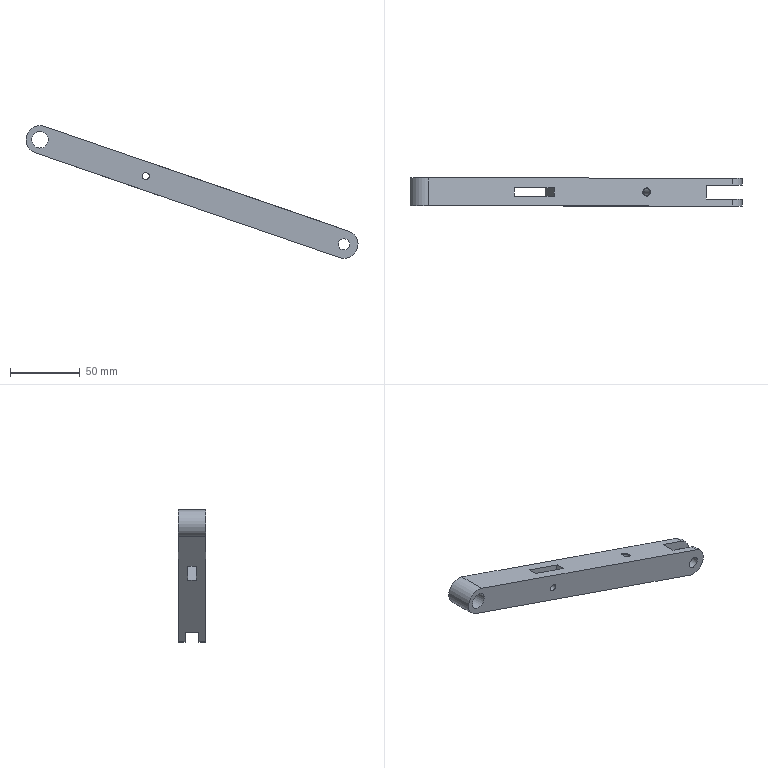Part | STEP file | 冲床-300配套压波_id682_x_t | 1 solid | 22 faces | box 237.457 x 20 x 94.916 mm | volume 85651 mm3 | plane 11 | cylinder 9 | cone 2 | commonest cylinder face diameters 5 x3 20 x3 8 x2 12 x1
STEP:
#1=CARTESIAN_POINT('',(2190.2,-5.,-445.371));
#2=VERTEX_POINT('',#1);
#3=CARTESIAN_POINT('',(2171.291,-5.,-438.856));
#4=VERTEX_POINT('',#3);
#5=CARTESIAN_POINT('',(2038.925,-5.,-393.255));
#6=DIRECTION('',(-0.9455,0.,0.3257));
#7=VECTOR('',#6,1.);
#8=LINE('',#5,#7);
#9=EDGE_CURVE('',#2,#4,#8,.T.);
#10=ORIENTED_EDGE('',*,*,#9,.F.);
#11=CARTESIAN_POINT('',(2190.2,-10.,-445.371));
#12=VERTEX_POINT('',#11);
#13=CARTESIAN_POINT('',(2190.2,-10.,-445.371));
#14=DIRECTION('',(0.,-1.,0.));
#15=VECTOR('',#14,1.);
#16=LINE('',#13,#15);
#17=EDGE_CURVE('',#2,#12,#16,.T.);
#18=ORIENTED_EDGE('',*,*,#17,.T.);
#19=CARTESIAN_POINT('',(1972.743,-10.,-370.455));
#20=VERTEX_POINT('',#19);
#21=CARTESIAN_POINT('',(1958.561,-10.,-365.569));
#22=DIRECTION('',(0.9455,0.,-0.3257));
#23=VECTOR('',#22,1.);
#24=LINE('',#21,#23);
#25=EDGE_CURVE('',#20,#12,#24,.T.);
#26=ORIENTED_EDGE('',*,*,#25,.F.);
#27=CARTESIAN_POINT('',(1972.743,10.,-370.455));
#28=VERTEX_POINT('',#27);
#29=CARTESIAN_POINT('',(1972.743,0.,-370.455));
#30=DIRECTION('',(0.,1.,0.));
#31=VECTOR('',#30,1.);
#32=LINE('',#29,#31);
#33=EDGE_CURVE('',#20,#28,#32,.T.);
#34=ORIENTED_EDGE('',*,*,#33,.T.);
#35=CARTESIAN_POINT('',(2190.2,10.,-445.371));
#36=VERTEX_POINT('',#35);
#37=CARTESIAN_POINT('',(1958.561,10.,-365.569));
#38=DIRECTION('',(0.9455,0.,-0.3257));
#39=VECTOR('',#38,1.);
#40=LINE('',#37,#39);
#41=EDGE_CURVE('',#28,#36,#40,.T.);
#42=ORIENTED_EDGE('',*,*,#41,.T.);
#43=CARTESIAN_POINT('',(2190.2,5.,-445.371));
#44=VERTEX_POINT('',#43);
#45=CARTESIAN_POINT('',(2190.2,-10.,-445.371));
#46=DIRECTION('',(0.,-1.,0.));
#47=VECTOR('',#46,1.);
#48=LINE('',#45,#47);
#49=EDGE_CURVE('',#36,#44,#48,.T.);
#50=ORIENTED_EDGE('',*,*,#49,.T.);
#51=CARTESIAN_POINT('',(2171.291,5.,-438.856));
#52=VERTEX_POINT('',#51);
#53=CARTESIAN_POINT('',(2038.925,5.,-393.255));
#54=DIRECTION('',(0.9455,0.,-0.3257));
#55=VECTOR('',#54,1.);
#56=LINE('',#53,#55);
#57=EDGE_CURVE('',#52,#44,#56,.T.);
#58=ORIENTED_EDGE('',*,*,#57,.F.);
#59=CARTESIAN_POINT('',(2171.291,-10.,-438.856));
#60=DIRECTION('',(0.,1.,0.));
#61=VECTOR('',#60,1.);
#62=LINE('',#59,#61);
#63=EDGE_CURVE('',#4,#52,#62,.T.);
#64=ORIENTED_EDGE('',*,*,#63,.F.);
#65=EDGE_LOOP('',(#10,#18,#26,#34,#42,#50,#58,#64));
#66=FACE_BOUND('',#65,.T.);
#67=CARTESIAN_POINT('',(2062.562,3.15,-401.398));
#68=VERTEX_POINT('',#67);
#69=CARTESIAN_POINT('',(2062.562,-3.15,-401.398));
#70=VERTEX_POINT('',#69);
#71=CARTESIAN_POINT('',(2062.562,-3.1,-401.398));
#72=DIRECTION('',(0.,-1.,0.));
#73=VECTOR('',#72,1.);
#74=LINE('',#71,#73);
#75=EDGE_CURVE('',#68,#70,#74,.T.);
#76=ORIENTED_EDGE('',*,*,#75,.F.);
#77=CARTESIAN_POINT('',(2034.198,3.15,-391.627));
#78=VERTEX_POINT('',#77);
#79=CARTESIAN_POINT('',(1977.47,3.15,-372.083));
#80=DIRECTION('',(0.9455,0.,-0.3257));
#81=VECTOR('',#80,1.);
#82=LINE('',#79,#81);
#83=EDGE_CURVE('',#78,#68,#82,.T.);
#84=ORIENTED_EDGE('',*,*,#83,.F.);
#85=CARTESIAN_POINT('',(2034.198,-3.15,-391.627));
#86=VERTEX_POINT('',#85);
#87=CARTESIAN_POINT('',(2034.198,-10.,-391.627));
#88=DIRECTION('',(0.,-1.,0.));
#89=VECTOR('',#88,1.);
#90=LINE('',#87,#89);
#91=EDGE_CURVE('',#78,#86,#90,.T.);
#92=ORIENTED_EDGE('',*,*,#91,.T.);
#93=CARTESIAN_POINT('',(1977.47,-3.15,-372.083));
#94=DIRECTION('',(-0.9455,0.,0.3257));
#95=VECTOR('',#94,1.);
#96=LINE('',#93,#95);
#97=EDGE_CURVE('',#70,#86,#96,.T.);
#98=ORIENTED_EDGE('',*,*,#97,.F.);
#99=EDGE_LOOP('',(#76,#84,#92,#98));
#100=FACE_BOUND('',#99,.T.);
#101=CARTESIAN_POINT('',(1958.561,-10.,-365.569));
#102=DIRECTION('',(0.3257,0.,0.9455));
#103=DIRECTION('',(0.9455,0.,-0.3257));
#104=AXIS2_PLACEMENT_3D('',#101,#102,#103);
#105=PLANE('',#104);
#106=ADVANCED_FACE('',(#66,#100),#105,.F.);
#107=CARTESIAN_POINT('',(2132.423,0.,-404.312));
#108=VERTEX_POINT('',#107);
#109=CARTESIAN_POINT('',(2135.259,0.,-405.289));
#110=DIRECTION('',(-0.3257,0.,-0.9455));
#111=DIRECTION('',(-0.9455,0.,0.3257));
#112=AXIS2_PLACEMENT_3D('',#109,#110,#111);
#113=CIRCLE('',#112,3.);
#114=EDGE_CURVE('',#108,#108,#113,.T.);
#115=ORIENTED_EDGE('',*,*,#114,.T.);
#116=EDGE_LOOP('',(#115));
#117=FACE_BOUND('',#116,.T.);
#118=CARTESIAN_POINT('',(2177.805,-5.,-419.947));
#119=VERTEX_POINT('',#118);
#120=CARTESIAN_POINT('',(2196.714,-5.,-426.461));
#121=VERTEX_POINT('',#120);
#122=CARTESIAN_POINT('',(2187.26,-5.,-423.204));
#123=DIRECTION('',(0.9455,0.,-0.3257));
#124=VECTOR('',#123,1.);
#125=LINE('',#122,#124);
#126=EDGE_CURVE('',#119,#121,#125,.T.);
#127=ORIENTED_EDGE('',*,*,#126,.F.);
#128=CARTESIAN_POINT('',(2177.805,5.,-419.947));
#129=VERTEX_POINT('',#128);
#130=CARTESIAN_POINT('',(2177.805,-10.,-419.947));
#131=DIRECTION('',(0.,-1.,0.));
#132=VECTOR('',#131,1.);
#133=LINE('',#130,#132);
#134=EDGE_CURVE('',#129,#119,#133,.T.);
#135=ORIENTED_EDGE('',*,*,#134,.F.);
#136=CARTESIAN_POINT('',(2196.714,5.,-426.461));
#137=VERTEX_POINT('',#136);
#138=CARTESIAN_POINT('',(2187.26,5.,-423.204));
#139=DIRECTION('',(-0.9455,0.,0.3257));
#140=VECTOR('',#139,1.);
#141=LINE('',#138,#140);
#142=EDGE_CURVE('',#137,#129,#141,.T.);
#143=ORIENTED_EDGE('',*,*,#142,.F.);
#144=CARTESIAN_POINT('',(2196.714,10.,-426.461));
#145=VERTEX_POINT('',#144);
#146=CARTESIAN_POINT('',(2196.714,-10.,-426.461));
#147=DIRECTION('',(0.,1.,0.));
#148=VECTOR('',#147,1.);
#149=LINE('',#146,#148);
#150=EDGE_CURVE('',#137,#145,#149,.T.);
#151=ORIENTED_EDGE('',*,*,#150,.T.);
#152=CARTESIAN_POINT('',(1979.257,10.,-351.545));
#153=VERTEX_POINT('',#152);
#154=CARTESIAN_POINT('',(2106.895,10.,-395.518));
#155=DIRECTION('',(-0.9455,0.,0.3257));
#156=VECTOR('',#155,1.);
#157=LINE('',#154,#156);
#158=EDGE_CURVE('',#145,#153,#157,.T.);
#159=ORIENTED_EDGE('',*,*,#158,.T.);
#160=CARTESIAN_POINT('',(1979.257,-10.,-351.545));
#161=VERTEX_POINT('',#160);
#162=CARTESIAN_POINT('',(1979.257,0.,-351.545));
#163=DIRECTION('',(0.,-1.,0.));
#164=VECTOR('',#163,1.);
#165=LINE('',#162,#164);
#166=EDGE_CURVE('',#153,#161,#165,.T.);
#167=ORIENTED_EDGE('',*,*,#166,.T.);
#168=CARTESIAN_POINT('',(2196.714,-10.,-426.461));
#169=VERTEX_POINT('',#168);
#170=CARTESIAN_POINT('',(2106.895,-10.,-395.518));
#171=DIRECTION('',(-0.9455,0.,0.3257));
#172=VECTOR('',#171,1.);
#173=LINE('',#170,#172);
#174=EDGE_CURVE('',#169,#161,#173,.T.);
#175=ORIENTED_EDGE('',*,*,#174,.F.);
#176=CARTESIAN_POINT('',(2196.714,-10.,-426.461));
#177=DIRECTION('',(0.,1.,0.));
#178=VECTOR('',#177,1.);
#179=LINE('',#176,#178);
#180=EDGE_CURVE('',#169,#121,#179,.T.);
#181=ORIENTED_EDGE('',*,*,#180,.T.);
#182=EDGE_LOOP('',(#127,#135,#143,#151,#159,#167,#175,#181));
#183=FACE_BOUND('',#182,.T.);
#184=CARTESIAN_POINT('',(2040.712,3.15,-372.717));
#185=VERTEX_POINT('',#184);
#186=CARTESIAN_POINT('',(2069.076,3.15,-382.489));
#187=VERTEX_POINT('',#186);
#188=CARTESIAN_POINT('',(2066.439,3.15,-381.58));
#189=DIRECTION('',(0.9455,0.,-0.3257));
#190=VECTOR('',#189,1.);
#191=LINE('',#188,#190);
#192=EDGE_CURVE('',#185,#187,#191,.T.);
#193=ORIENTED_EDGE('',*,*,#192,.T.);
#194=CARTESIAN_POINT('',(2069.076,-3.15,-382.489));
#195=VERTEX_POINT('',#194);
#196=CARTESIAN_POINT('',(2069.076,-10.,-382.489));
#197=DIRECTION('',(0.,-1.,0.));
#198=VECTOR('',#197,1.);
#199=LINE('',#196,#198);
#200=EDGE_CURVE('',#187,#195,#199,.T.);
#201=ORIENTED_EDGE('',*,*,#200,.T.);
#202=CARTESIAN_POINT('',(2040.712,-3.15,-372.717));
#203=VERTEX_POINT('',#202);
#204=CARTESIAN_POINT('',(2066.439,-3.15,-381.58));
#205=DIRECTION('',(-0.9455,0.,0.3257));
#206=VECTOR('',#205,1.);
#207=LINE('',#204,#206);
#208=EDGE_CURVE('',#195,#203,#207,.T.);
#209=ORIENTED_EDGE('',*,*,#208,.T.);
#210=CARTESIAN_POINT('',(2040.712,-10.,-372.717));
#211=DIRECTION('',(0.,1.,0.));
#212=VECTOR('',#211,1.);
#213=LINE('',#210,#212);
#214=EDGE_CURVE('',#203,#185,#213,.T.);
#215=ORIENTED_EDGE('',*,*,#214,.T.);
#216=EDGE_LOOP('',(#193,#201,#209,#215));
#217=FACE_BOUND('',#216,.T.);
#218=CARTESIAN_POINT('',(2106.895,-10.,-395.518));
#219=DIRECTION('',(-0.3257,0.,-0.9455));
#220=DIRECTION('',(-0.9455,0.,0.3257));
#221=AXIS2_PLACEMENT_3D('',#218,#219,#220);
#222=PLANE('',#221);
#223=ADVANCED_FACE('',(#117,#183,#217),#222,.F.);
#224=CARTESIAN_POINT('',(2050.584,-3.15,-384.79));
#225=VERTEX_POINT('',#224);
#226=CARTESIAN_POINT('',(2051.637,-3.15,-387.058));
#227=DIRECTION('',(0.,-1.,0.));
#228=DIRECTION('',(-0.4213,0.,0.9069));
#229=AXIS2_PLACEMENT_3D('',#226,#227,#228);
#230=CIRCLE('',#229,2.5);
#231=EDGE_CURVE('',#225,#225,#230,.T.);
#232=ORIENTED_EDGE('',*,*,#231,.F.);
#233=EDGE_LOOP('',(#232));
#234=FACE_BOUND('',#233,.T.);
#235=CARTESIAN_POINT('',(2050.064,-10.,-389.));
#236=VERTEX_POINT('',#235);
#237=CARTESIAN_POINT('',(2051.637,-10.,-387.058));
#238=DIRECTION('',(0.,1.,0.));
#239=DIRECTION('',(-0.6294,0.,-0.777));
#240=AXIS2_PLACEMENT_3D('',#237,#238,#239);
#241=CIRCLE('',#240,2.5);
#242=EDGE_CURVE('',#236,#236,#241,.T.);
#243=ORIENTED_EDGE('',*,*,#242,.F.);
#244=EDGE_LOOP('',(#243));
#245=FACE_BOUND('',#244,.T.);
#246=CARTESIAN_POINT('',(2051.637,-45.,-387.058));
#247=DIRECTION('',(0.,1.,0.));
#248=DIRECTION('',(0.6294,0.,0.777));
#249=AXIS2_PLACEMENT_3D('',#246,#247,#248);
#250=CYLINDRICAL_SURFACE('',#249,2.5);
#251=ADVANCED_FACE('',(#234,#245),#250,.F.);
#252=ORIENTED_EDGE('',*,*,#150,.F.);
#253=CARTESIAN_POINT('',(2193.457,5.,-435.916));
#254=DIRECTION('',(0.,1.,0.));
#255=DIRECTION('',(-0.3257,0.,-0.9455));
#256=AXIS2_PLACEMENT_3D('',#253,#254,#255);
#257=CIRCLE('',#256,10.);
#258=EDGE_CURVE('',#137,#44,#257,.T.);
#259=ORIENTED_EDGE('',*,*,#258,.T.);
#260=ORIENTED_EDGE('',*,*,#49,.F.);
#261=CARTESIAN_POINT('',(2193.457,10.,-435.916));
#262=DIRECTION('',(0.,1.,0.));
#263=DIRECTION('',(-0.3257,0.,-0.9455));
#264=AXIS2_PLACEMENT_3D('',#261,#262,#263);
#265=CIRCLE('',#264,10.);
#266=EDGE_CURVE('',#145,#36,#265,.T.);
#267=ORIENTED_EDGE('',*,*,#266,.F.);
#268=EDGE_LOOP('',(#252,#259,#260,#267));
#269=FACE_OUTER_BOUND('',#268,.T.);
#270=CARTESIAN_POINT('',(2193.457,-10.,-435.916));
#271=DIRECTION('',(0.,1.,0.));
#272=DIRECTION('',(0.3257,0.,0.9455));
#273=AXIS2_PLACEMENT_3D('',#270,#271,#272);
#274=CYLINDRICAL_SURFACE('',#273,10.);
#275=ADVANCED_FACE('',(#269),#274,.T.);
#276=ORIENTED_EDGE('',*,*,#17,.F.);
#277=CARTESIAN_POINT('',(2193.457,-5.,-435.916));
#278=DIRECTION('',(0.,-1.,0.));
#279=DIRECTION('',(0.3257,0.,0.9455));
#280=AXIS2_PLACEMENT_3D('',#277,#278,#279);
#281=CIRCLE('',#280,10.);
#282=EDGE_CURVE('',#2,#121,#281,.T.);
#283=ORIENTED_EDGE('',*,*,#282,.T.);
#284=ORIENTED_EDGE('',*,*,#180,.F.);
#285=CARTESIAN_POINT('',(2193.457,-10.,-435.916));
#286=DIRECTION('',(0.,-1.,0.));
#287=DIRECTION('',(-0.3257,0.,-0.9455));
#288=AXIS2_PLACEMENT_3D('',#285,#286,#287);
#289=CIRCLE('',#288,10.);
#290=EDGE_CURVE('',#12,#169,#289,.T.);
#291=ORIENTED_EDGE('',*,*,#290,.F.);
#292=EDGE_LOOP('',(#276,#283,#284,#291));
#293=FACE_OUTER_BOUND('',#292,.T.);
#294=CARTESIAN_POINT('',(2193.457,-10.,-435.916));
#295=DIRECTION('',(0.,1.,0.));
#296=DIRECTION('',(0.3257,0.,0.9455));
#297=AXIS2_PLACEMENT_3D('',#294,#295,#296);
#298=CYLINDRICAL_SURFACE('',#297,10.);
#299=ADVANCED_FACE('',(#293),#298,.T.);
#300=CARTESIAN_POINT('',(2192.154,-10.,-439.698));
#301=VERTEX_POINT('',#300);
#302=CARTESIAN_POINT('',(2193.457,-10.,-435.916));
#303=DIRECTION('',(0.,1.,0.));
#304=DIRECTION('',(-0.3257,0.,-0.9455));
#305=AXIS2_PLACEMENT_3D('',#302,#303,#304);
#306=CIRCLE('',#305,4.);
#307=EDGE_CURVE('',#301,#301,#306,.T.);
#308=ORIENTED_EDGE('',*,*,#307,.F.);
#309=EDGE_LOOP('',(#308));
#310=FACE_BOUND('',#309,.T.);
#311=CARTESIAN_POINT('',(2194.76,-5.,-432.134));
#312=VERTEX_POINT('',#311);
#313=CARTESIAN_POINT('',(2193.457,-5.,-435.916));
#314=DIRECTION('',(0.,-1.,0.));
#315=DIRECTION('',(0.3257,0.,0.9455));
#316=AXIS2_PLACEMENT_3D('',#313,#314,#315);
#317=CIRCLE('',#316,4.);
#318=EDGE_CURVE('',#312,#312,#317,.T.);
#319=ORIENTED_EDGE('',*,*,#318,.F.);
#320=EDGE_LOOP('',(#319));
#321=FACE_BOUND('',#320,.T.);
#322=CARTESIAN_POINT('',(2193.457,-10.,-435.916));
#323=DIRECTION('',(0.,1.,0.));
#324=DIRECTION('',(0.3257,0.,0.9455));
#325=AXIS2_PLACEMENT_3D('',#322,#323,#324);
#326=CYLINDRICAL_SURFACE('',#325,4.);
#327=ADVANCED_FACE('',(#310,#321),#326,.F.);
#328=CARTESIAN_POINT('',(2192.154,10.,-439.698));
#329=VERTEX_POINT('',#328);
#330=CARTESIAN_POINT('',(2193.457,10.,-435.916));
#331=DIRECTION('',(0.,-1.,0.));
#332=DIRECTION('',(-0.3257,0.,-0.9455));
#333=AXIS2_PLACEMENT_3D('',#330,#331,#332);
#334=CIRCLE('',#333,4.);
#335=EDGE_CURVE('',#329,#329,#334,.T.);
#336=ORIENTED_EDGE('',*,*,#335,.F.);
#337=EDGE_LOOP('',(#336));
#338=FACE_BOUND('',#337,.T.);
#339=CARTESIAN_POINT('',(2192.154,5.,-439.698));
#340=VERTEX_POINT('',#339);
#341=CARTESIAN_POINT('',(2193.457,5.,-435.916));
#342=DIRECTION('',(0.,1.,0.));
#343=DIRECTION('',(-0.3257,0.,-0.9455));
#344=AXIS2_PLACEMENT_3D('',#341,#342,#343);
#345=CIRCLE('',#344,4.);
#346=EDGE_CURVE('',#340,#340,#345,.T.);
#347=ORIENTED_EDGE('',*,*,#346,.F.);
#348=EDGE_LOOP('',(#347));
#349=FACE_BOUND('',#348,.T.);
#350=CARTESIAN_POINT('',(2193.457,-10.,-435.916));
#351=DIRECTION('',(0.,1.,0.));
#352=DIRECTION('',(0.3257,0.,0.9455));
#353=AXIS2_PLACEMENT_3D('',#350,#351,#352);
#354=CYLINDRICAL_SURFACE('',#353,4.);
#355=ADVANCED_FACE('',(#338,#349),#354,.F.);
#356=ORIENTED_EDGE('',*,*,#242,.T.);
#357=EDGE_LOOP('',(#356));
#358=FACE_BOUND('',#357,.T.);
#359=CARTESIAN_POINT('',(1976.,-10.,-367.));
#360=VERTEX_POINT('',#359);
#361=CARTESIAN_POINT('',(1976.,-10.,-361.));
#362=DIRECTION('',(0.,1.,0.));
#363=DIRECTION('',(0.,0.,-1.));
#364=AXIS2_PLACEMENT_3D('',#361,#362,#363);
#365=CIRCLE('',#364,6.);
#366=EDGE_CURVE('',#360,#360,#365,.T.);
#367=ORIENTED_EDGE('',*,*,#366,.T.);
#368=EDGE_LOOP('',(#367));
#369=FACE_BOUND('',#368,.T.);
#370=ORIENTED_EDGE('',*,*,#307,.T.);
#371=EDGE_LOOP('',(#370));
#372=FACE_BOUND('',#371,.T.);
#373=ORIENTED_EDGE('',*,*,#25,.T.);
#374=ORIENTED_EDGE('',*,*,#290,.T.);
#375=ORIENTED_EDGE('',*,*,#174,.T.);
#376=CARTESIAN_POINT('',(1976.,-10.,-361.));
#377=DIRECTION('',(0.,-1.,0.));
#378=DIRECTION('',(0.4213,0.,-0.9069));
#379=AXIS2_PLACEMENT_3D('',#376,#377,#378);
#380=CIRCLE('',#379,10.);
#381=EDGE_CURVE('',#161,#20,#380,.T.);
#382=ORIENTED_EDGE('',*,*,#381,.T.);
#383=EDGE_LOOP('',(#373,#374,#375,#382));
#384=FACE_BOUND('',#383,.T.);
#385=CARTESIAN_POINT('',(184.727,-10.,507.573));
#386=DIRECTION('',(0.,-1.,0.));
#387=DIRECTION('',(-0.3257,0.,-0.9455));
#388=AXIS2_PLACEMENT_3D('',#385,#386,#387);
#389=PLANE('',#388);
#390=ADVANCED_FACE('',(#358,#369,#372,#384),#389,.T.);
#391=CARTESIAN_POINT('',(2050.064,10.,-389.));
#392=VERTEX_POINT('',#391);
#393=CARTESIAN_POINT('',(2051.637,10.,-387.058));
#394=DIRECTION('',(0.,1.,0.));
#395=DIRECTION('',(-0.6294,0.,-0.777));
#396=AXIS2_PLACEMENT_3D('',#393,#394,#395);
#397=CIRCLE('',#396,2.5);
#398=EDGE_CURVE('',#392,#392,#397,.T.);
#399=ORIENTED_EDGE('',*,*,#398,.F.);
#400=EDGE_LOOP('',(#399));
#401=FACE_BOUND('',#400,.T.);
#402=CARTESIAN_POINT('',(1976.,10.,-367.));
#403=VERTEX_POINT('',#402);
#404=CARTESIAN_POINT('',(1976.,10.,-361.));
#405=DIRECTION('',(0.,1.,0.));
#406=DIRECTION('',(0.,0.,-1.));
#407=AXIS2_PLACEMENT_3D('',#404,#405,#406);
#408=CIRCLE('',#407,6.);
#409=EDGE_CURVE('',#403,#403,#408,.T.);
#410=ORIENTED_EDGE('',*,*,#409,.F.);
#411=EDGE_LOOP('',(#410));
#412=FACE_BOUND('',#411,.T.);
#413=ORIENTED_EDGE('',*,*,#335,.T.);
#414=EDGE_LOOP('',(#413));
#415=FACE_BOUND('',#414,.T.);
#416=ORIENTED_EDGE('',*,*,#266,.T.);
#417=ORIENTED_EDGE('',*,*,#41,.F.);
#418=CARTESIAN_POINT('',(1976.,10.,-361.));
#419=DIRECTION('',(0.,1.,0.));
#420=DIRECTION('',(0.4213,0.,-0.9069));
#421=AXIS2_PLACEMENT_3D('',#418,#419,#420);
#422=CIRCLE('',#421,10.);
#423=EDGE_CURVE('',#28,#153,#422,.T.);
#424=ORIENTED_EDGE('',*,*,#423,.T.);
#425=ORIENTED_EDGE('',*,*,#158,.F.);
#426=EDGE_LOOP('',(#416,#417,#424,#425));
#427=FACE_BOUND('',#426,.T.);
#428=CARTESIAN_POINT('',(184.727,10.,507.573));
#429=DIRECTION('',(0.,-1.,0.));
#430=DIRECTION('',(-0.3257,0.,-0.9455));
#431=AXIS2_PLACEMENT_3D('',#428,#429,#430);
#432=PLANE('',#431);
#433=ADVANCED_FACE('',(#401,#412,#415,#427),#432,.F.);
#434=ORIENTED_EDGE('',*,*,#423,.F.);
#435=ORIENTED_EDGE('',*,*,#33,.F.);
#436=ORIENTED_EDGE('',*,*,#381,.F.);
#437=ORIENTED_EDGE('',*,*,#166,.F.);
#438=EDGE_LOOP('',(#434,#435,#436,#437));
#439=FACE_OUTER_BOUND('',#438,.T.);
#440=CARTESIAN_POINT('',(1976.,-2.,-361.));
#441=DIRECTION('',(0.,-1.,0.));
#442=DIRECTION('',(0.4213,0.,-0.9069));
#443=AXIS2_PLACEMENT_3D('',#440,#441,#442);
#444=CYLINDRICAL_SURFACE('',#443,10.);
#445=ADVANCED_FACE('',(#439),#444,.T.);
#446=ORIENTED_EDGE('',*,*,#366,.F.);
#447=EDGE_LOOP('',(#446));
#448=FACE_BOUND('',#447,.T.);
#449=ORIENTED_EDGE('',*,*,#409,.T.);
#450=EDGE_LOOP('',(#449));
#451=FACE_BOUND('',#450,.T.);
#452=CARTESIAN_POINT('',(1976.,32.85,-361.));
#453=DIRECTION('',(0.,-1.,0.));
#454=DIRECTION('',(-0.3257,0.,-0.9455));
#455=AXIS2_PLACEMENT_3D('',#452,#453,#454);
#456=CYLINDRICAL_SURFACE('',#455,6.);
#457=ADVANCED_FACE('',(#448,#451),#456,.F.);
#458=ORIENTED_EDGE('',*,*,#63,.T.);
#459=CARTESIAN_POINT('',(2184.319,5.,-401.038));
#460=DIRECTION('',(0.3257,0.,0.9455));
#461=VECTOR('',#460,1.);
#462=LINE('',#459,#461);
#463=EDGE_CURVE('',#52,#129,#462,.T.);
#464=ORIENTED_EDGE('',*,*,#463,.T.);
#465=ORIENTED_EDGE('',*,*,#134,.T.);
#466=CARTESIAN_POINT('',(2184.319,-5.,-401.038));
#467=DIRECTION('',(0.3257,0.,0.9455));
#468=VECTOR('',#467,1.);
#469=LINE('',#466,#468);
#470=EDGE_CURVE('',#4,#119,#469,.T.);
#471=ORIENTED_EDGE('',*,*,#470,.F.);
#472=EDGE_LOOP('',(#458,#464,#465,#471));
#473=FACE_OUTER_BOUND('',#472,.T.);
#474=CARTESIAN_POINT('',(2184.319,5.,-401.038));
#475=DIRECTION('',(0.9455,0.,-0.3257));
#476=DIRECTION('',(-0.3257,0.,-0.9455));
#477=AXIS2_PLACEMENT_3D('',#474,#475,#476);
#478=PLANE('',#477);
#479=ADVANCED_FACE('',(#473),#478,.T.);
#480=ORIENTED_EDGE('',*,*,#318,.T.);
#481=EDGE_LOOP('',(#480));
#482=FACE_BOUND('',#481,.T.);
#483=ORIENTED_EDGE('',*,*,#9,.T.);
#484=ORIENTED_EDGE('',*,*,#470,.T.);
#485=ORIENTED_EDGE('',*,*,#126,.T.);
#486=ORIENTED_EDGE('',*,*,#282,.F.);
#487=EDGE_LOOP('',(#483,#484,#485,#486));
#488=FACE_BOUND('',#487,.T.);
#489=CARTESIAN_POINT('',(2184.319,-5.,-401.038));
#490=DIRECTION('',(0.,1.,0.));
#491=DIRECTION('',(0.3257,0.,0.9455));
#492=AXIS2_PLACEMENT_3D('',#489,#490,#491);
#493=PLANE('',#492);
#494=ADVANCED_FACE('',(#482,#488),#493,.T.);
#495=ORIENTED_EDGE('',*,*,#346,.T.);
#496=EDGE_LOOP('',(#495));
#497=FACE_BOUND('',#496,.T.);
#498=ORIENTED_EDGE('',*,*,#57,.T.);
#499=ORIENTED_EDGE('',*,*,#258,.F.);
#500=ORIENTED_EDGE('',*,*,#142,.T.);
#501=ORIENTED_EDGE('',*,*,#463,.F.);
#502=EDGE_LOOP('',(#498,#499,#500,#501));
#503=FACE_BOUND('',#502,.T.);
#504=CARTESIAN_POINT('',(2223.333,5.,-414.478));
#505=DIRECTION('',(0.,-1.,0.));
#506=DIRECTION('',(-0.3257,0.,-0.9455));
#507=AXIS2_PLACEMENT_3D('',#504,#505,#506);
#508=PLANE('',#507);
#509=ADVANCED_FACE('',(#497,#503),#508,.T.);
#510=CARTESIAN_POINT('',(2052.69,3.15,-389.325));
#511=VERTEX_POINT('',#510);
#512=CARTESIAN_POINT('',(2051.637,3.15,-387.058));
#513=DIRECTION('',(0.,1.,0.));
#514=DIRECTION('',(0.4213,0.,-0.9069));
#515=AXIS2_PLACEMENT_3D('',#512,#513,#514);
#516=CIRCLE('',#515,2.5);
#517=EDGE_CURVE('',#511,#511,#516,.T.);
#518=ORIENTED_EDGE('',*,*,#517,.F.);
#519=EDGE_LOOP('',(#518));
#520=FACE_BOUND('',#519,.T.);
#521=ORIENTED_EDGE('',*,*,#398,.T.);
#522=EDGE_LOOP('',(#521));
#523=FACE_BOUND('',#522,.T.);
#524=CARTESIAN_POINT('',(2051.637,-45.,-387.058));
#525=DIRECTION('',(0.,1.,0.));
#526=DIRECTION('',(0.6294,0.,0.777));
#527=AXIS2_PLACEMENT_3D('',#524,#525,#526);
#528=CYLINDRICAL_SURFACE('',#527,2.5);
#529=ADVANCED_FACE('',(#520,#523),#528,.F.);
#530=CARTESIAN_POINT('',(2128.987,0.,-415.821));
#531=VERTEX_POINT('',#530);
#532=CARTESIAN_POINT('',(2131.35,0.,-416.635));
#533=DIRECTION('',(0.3257,0.,0.9455));
#534=DIRECTION('',(-0.9455,0.,0.3257));
#535=AXIS2_PLACEMENT_3D('',#532,#533,#534);
#536=CIRCLE('',#535,2.5);
#537=EDGE_CURVE('',#531,#531,#536,.T.);
#538=ORIENTED_EDGE('',*,*,#537,.T.);
#539=EDGE_LOOP('',(#538));
#540=FACE_BOUND('',#539,.T.);
#541=CARTESIAN_POINT('',(2130.861,0.,-418.055));
#542=VERTEX_POINT('',#541);
#543=VERTEX_LOOP('',#542);
#544=FACE_BOUND('',#543,.T.);
#545=CARTESIAN_POINT('',(2131.35,0.,-416.635));
#546=DIRECTION('',(0.3257,0.,0.9455));
#547=DIRECTION('',(0.9455,0.,-0.3257));
#548=AXIS2_PLACEMENT_3D('',#545,#546,#547);
#549=CONICAL_SURFACE('',#548,2.5,59.);
#550=ADVANCED_FACE('',(#540,#544),#549,.F.);
#551=CARTESIAN_POINT('',(2132.733,0.,-404.948));
#552=VERTEX_POINT('',#551);
#553=CARTESIAN_POINT('',(2135.096,0.,-405.762));
#554=DIRECTION('',(0.3257,0.,0.9455));
#555=DIRECTION('',(-0.9455,0.,0.3257));
#556=AXIS2_PLACEMENT_3D('',#553,#554,#555);
#557=CIRCLE('',#556,2.5);
#558=EDGE_CURVE('',#552,#552,#557,.T.);
#559=ORIENTED_EDGE('',*,*,#558,.T.);
#560=EDGE_LOOP('',(#559));
#561=FACE_BOUND('',#560,.T.);
#562=ORIENTED_EDGE('',*,*,#537,.F.);
#563=EDGE_LOOP('',(#562));
#564=FACE_BOUND('',#563,.T.);
#565=CARTESIAN_POINT('',(2135.259,0.,-405.289));
#566=DIRECTION('',(-0.3257,0.,-0.9455));
#567=DIRECTION('',(-0.9455,0.,0.3257));
#568=AXIS2_PLACEMENT_3D('',#565,#566,#567);
#569=CYLINDRICAL_SURFACE('',#568,2.5);
#570=ADVANCED_FACE('',(#561,#564),#569,.F.);
#571=ORIENTED_EDGE('',*,*,#558,.F.);
#572=EDGE_LOOP('',(#571));
#573=FACE_BOUND('',#572,.T.);
#574=ORIENTED_EDGE('',*,*,#114,.F.);
#575=EDGE_LOOP('',(#574));
#576=FACE_BOUND('',#575,.T.);
#577=CARTESIAN_POINT('',(2135.259,0.,-405.289));
#578=DIRECTION('',(0.3257,0.,0.9455));
#579=DIRECTION('',(0.9455,0.,-0.3257));
#580=AXIS2_PLACEMENT_3D('',#577,#578,#579);
#581=CONICAL_SURFACE('',#580,3.,45.);
#582=ADVANCED_FACE('',(#573,#576),#581,.F.);
#583=ORIENTED_EDGE('',*,*,#517,.T.);
#584=EDGE_LOOP('',(#583));
#585=FACE_BOUND('',#584,.T.);
#586=ORIENTED_EDGE('',*,*,#192,.F.);
#587=CARTESIAN_POINT('',(2034.489,3.15,-390.781));
#588=DIRECTION('',(-0.3257,0.,-0.9455));
#589=VECTOR('',#588,1.);
#590=LINE('',#587,#589);
#591=EDGE_CURVE('',#185,#78,#590,.T.);
#592=ORIENTED_EDGE('',*,*,#591,.T.);
#593=ORIENTED_EDGE('',*,*,#83,.T.);
#594=CARTESIAN_POINT('',(2062.853,3.15,-400.553));
#595=DIRECTION('',(0.3257,0.,0.9455));
#596=VECTOR('',#595,1.);
#597=LINE('',#594,#596);
#598=EDGE_CURVE('',#68,#187,#597,.T.);
#599=ORIENTED_EDGE('',*,*,#598,.T.);
#600=EDGE_LOOP('',(#586,#592,#593,#599));
#601=FACE_BOUND('',#600,.T.);
#602=CARTESIAN_POINT('',(2060.215,3.15,-399.644));
#603=DIRECTION('',(0.,-1.,0.));
#604=DIRECTION('',(0.1921,0.,-0.9814));
#605=AXIS2_PLACEMENT_3D('',#602,#603,#604);
#606=PLANE('',#605);
#607=ADVANCED_FACE('',(#585,#601),#606,.T.);
#608=ORIENTED_EDGE('',*,*,#231,.T.);
#609=EDGE_LOOP('',(#608));
#610=FACE_BOUND('',#609,.T.);
#611=ORIENTED_EDGE('',*,*,#97,.T.);
#612=CARTESIAN_POINT('',(2034.489,-3.15,-390.781));
#613=DIRECTION('',(0.3257,0.,0.9455));
#614=VECTOR('',#613,1.);
#615=LINE('',#612,#614);
#616=EDGE_CURVE('',#86,#203,#615,.T.);
#617=ORIENTED_EDGE('',*,*,#616,.T.);
#618=ORIENTED_EDGE('',*,*,#208,.F.);
#619=CARTESIAN_POINT('',(2062.853,-3.15,-400.553));
#620=DIRECTION('',(-0.3257,0.,-0.9455));
#621=VECTOR('',#620,1.);
#622=LINE('',#619,#621);
#623=EDGE_CURVE('',#195,#70,#622,.T.);
#624=ORIENTED_EDGE('',*,*,#623,.T.);
#625=EDGE_LOOP('',(#611,#617,#618,#624));
#626=FACE_BOUND('',#625,.T.);
#627=CARTESIAN_POINT('',(2060.215,-3.15,-399.644));
#628=DIRECTION('',(0.,1.,0.));
#629=DIRECTION('',(-0.1921,0.,0.9814));
#630=AXIS2_PLACEMENT_3D('',#627,#628,#629);
#631=PLANE('',#630);
#632=ADVANCED_FACE('',(#610,#626),#631,.T.);
#633=ORIENTED_EDGE('',*,*,#616,.F.);
#634=ORIENTED_EDGE('',*,*,#91,.F.);
#635=ORIENTED_EDGE('',*,*,#591,.F.);
#636=ORIENTED_EDGE('',*,*,#214,.F.);
#637=EDGE_LOOP('',(#633,#634,#635,#636));
#638=FACE_OUTER_BOUND('',#637,.T.);
#639=CARTESIAN_POINT('',(2036.546,-3.1,-384.811));
#640=DIRECTION('',(-0.9455,0.,0.3257));
#641=DIRECTION('',(0.3257,0.,0.9455));
#642=AXIS2_PLACEMENT_3D('',#639,#640,#641);
#643=PLANE('',#642);
#644=ADVANCED_FACE('',(#638),#643,.F.);
#645=ORIENTED_EDGE('',*,*,#598,.F.);
#646=ORIENTED_EDGE('',*,*,#75,.T.);
#647=ORIENTED_EDGE('',*,*,#623,.F.);
#648=ORIENTED_EDGE('',*,*,#200,.F.);
#649=EDGE_LOOP('',(#645,#646,#647,#648));
#650=FACE_OUTER_BOUND('',#649,.T.);
#651=CARTESIAN_POINT('',(2064.91,-3.1,-394.583));
#652=DIRECTION('',(-0.9455,0.,0.3257));
#653=DIRECTION('',(0.3257,0.,0.9455));
#654=AXIS2_PLACEMENT_3D('',#651,#652,#653);
#655=PLANE('',#654);
#656=ADVANCED_FACE('',(#650),#655,.T.);
#657=CLOSED_SHELL('',(#106,#223,#251,#275,#299,#327,#355,#390,#433,#445,#457,#479,#494,#509,#529,#550,#570,#582,#607,#632,#644,#656));
#658=MANIFOLD_SOLID_BREP('',#657);
#659=(LENGTH_UNIT()NAMED_UNIT(*)SI_UNIT(.MILLI.,.METRE.));
#660=UNCERTAINTY_MEASURE_WITH_UNIT(LENGTH_MEASURE(0.00002),#659,'','');
#661=(NAMED_UNIT(*)PLANE_ANGLE_UNIT()SI_UNIT($,.RADIAN.));
#662=PLANE_ANGLE_MEASURE_WITH_UNIT(PLANE_ANGLE_MEASURE(0.01745),#661);
#663=DIMENSIONAL_EXPONENTS(0.,0.,0.,0.,0.,0.,0.);
#664=(CONVERSION_BASED_UNIT('DEGREE',#662)NAMED_UNIT(#663)PLANE_ANGLE_UNIT());
#665=(NAMED_UNIT(*)SI_UNIT($,.STERADIAN.)SOLID_ANGLE_UNIT());
#666=(GEOMETRIC_REPRESENTATION_CONTEXT(3)GLOBAL_UNCERTAINTY_ASSIGNED_CONTEXT((#660))GLOBAL_UNIT_ASSIGNED_CONTEXT((#659,#664,#665))REPRESENTATION_CONTEXT('',''));
#667=ADVANCED_BREP_SHAPE_REPRESENTATION('',(#658),#666);